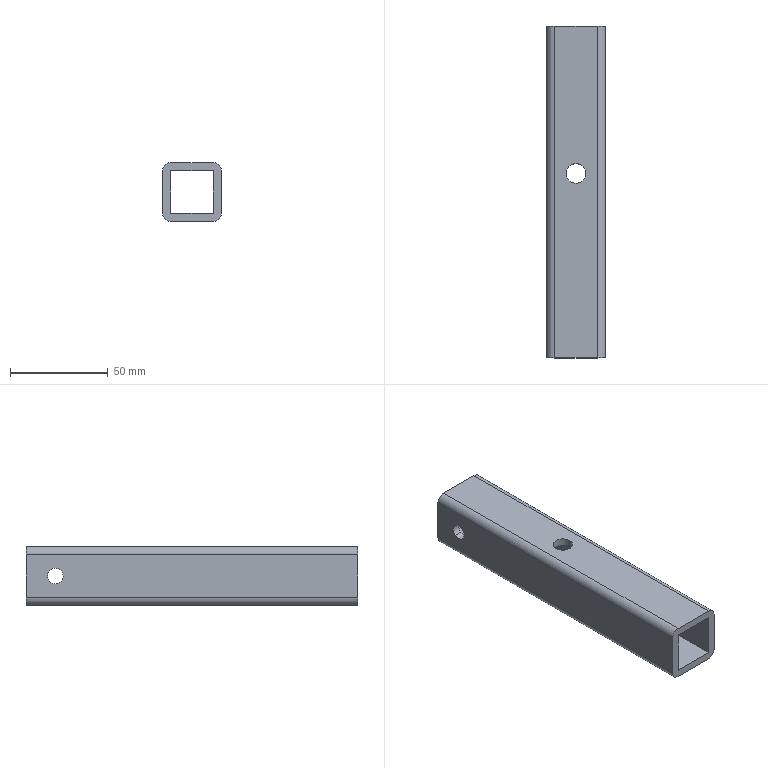Part | NX | features LINKED_BODY 2, SUBTRACT 2, BLEND 1, DATUM_CSYS 1, EXTRACT_DATUM_PLANE 1, EXTRUDE 1, SHELL 1, SKETCH 1 | 1 solid | 20 faces | volume 67348 mm3 | plane 10 | cylinder 10 | commonest cylinder face diameters 8 x8 10.051 x2